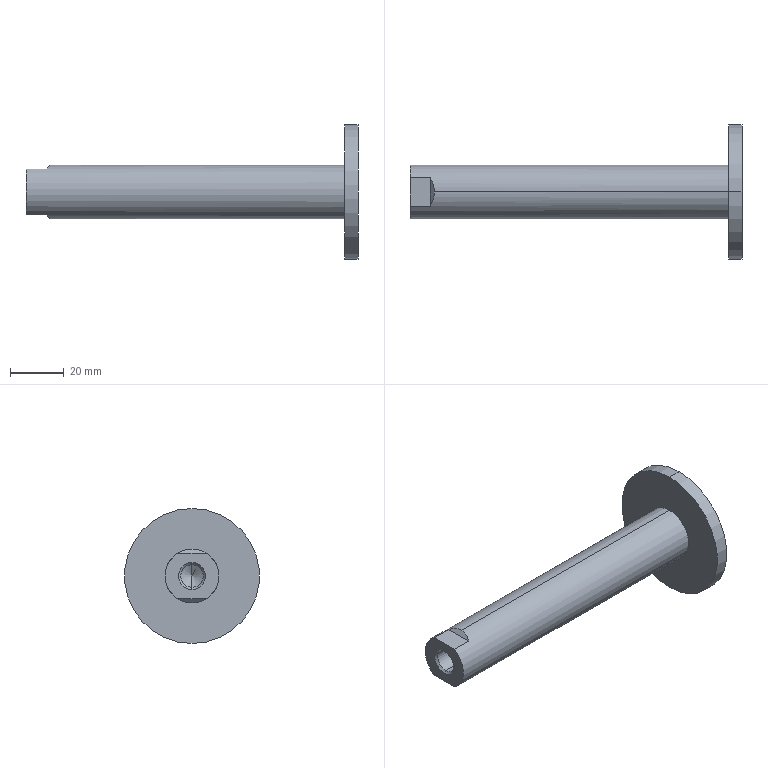Part | STEP file | _CDQ2A50-100-D-A93(0_0)_CYROD.stp | 1 solid | 17 faces | box 123 x 50 x 50 mm | volume 45835 mm3 | plane 7 | cylinder 6 | cone 4 | commonest cylinder face diameters 8.376 x2 20 x2 50 x2
STEP:
#1=CARTESIAN_POINT('',(0.,0.,0.));
#2=DIRECTION('',(0.,0.,1.));
#3=DIRECTION('',(1.,0.,0.));
#4=AXIS2_PLACEMENT_3D('',#1,#2,#3);
#5=CARTESIAN_POINT('',(7.,0.,4.188));
#6=VERTEX_POINT('',#5);
#7=CARTESIAN_POINT('',(7.,0.,-4.188));
#8=VERTEX_POINT('',#7);
#9=CARTESIAN_POINT('',(7.,0.,0.));
#10=DIRECTION('',(1.,0.,0.));
#11=DIRECTION('',(0.,0.,-1.));
#12=AXIS2_PLACEMENT_3D('',#9,#10,#11);
#13=CIRCLE('',#12,4.188);
#14=CARTESIAN_POINT('',(8.418,0.,0.));
#15=DIRECTION('',(-1.,0.,0.));
#16=DIRECTION('',(0.,0.,1.));
#17=AXIS2_PLACEMENT_3D('',#14,#15,#16);
#18=CONICAL_SURFACE('',#17,1.732,1.047);
#19=CARTESIAN_POINT('',(9.425,1.418));
#20=DIRECTION('',(-1.,0.));
#21=VECTOR('',#20,1.);
#22=LINE('',#19,#21);
#23=(GEOMETRIC_REPRESENTATION_CONTEXT(2)PARAMETRIC_REPRESENTATION_CONTEXT()REPRESENTATION_CONTEXT('',''));
#24=DEFINITIONAL_REPRESENTATION('',(#22),#23);
#25=PCURVE('',#18,#24);
#26=CARTESIAN_POINT('',(115.,0.,0.));
#27=DIRECTION('',(-1.,0.,0.));
#28=DIRECTION('',(0.,0.,-1.));
#29=AXIS2_PLACEMENT_3D('',#26,#27,#28);
#30=CYLINDRICAL_SURFACE('',#29,4.188);
#31=CARTESIAN_POINT('',(6.283,108.));
#32=DIRECTION('',(-1.,0.));
#33=VECTOR('',#32,1.);
#34=LINE('',#31,#33);
#35=(GEOMETRIC_REPRESENTATION_CONTEXT(2)PARAMETRIC_REPRESENTATION_CONTEXT()REPRESENTATION_CONTEXT('',''));
#36=DEFINITIONAL_REPRESENTATION('',(#34),#35);
#37=PCURVE('',#30,#36);
#38=SURFACE_CURVE('',#13,(#25,#37),.PCURVE_S1.);
#39=EDGE_CURVE('',#6,#8,#38,.T.);
#40=ORIENTED_EDGE('',*,*,#39,.T.);
#41=CARTESIAN_POINT('',(9.418,0.,0.));
#42=VERTEX_POINT('',#41);
#43=CARTESIAN_POINT('',(8.418,0.,-1.732));
#44=DIRECTION('',(-0.5,0.,-0.866));
#45=VECTOR('',#44,1.);
#46=LINE('',#43,#45);
#47=CARTESIAN_POINT('',(3.142,0.));
#48=DIRECTION('',(0.,1.));
#49=VECTOR('',#48,1.);
#50=LINE('',#47,#49);
#51=(GEOMETRIC_REPRESENTATION_CONTEXT(2)PARAMETRIC_REPRESENTATION_CONTEXT()REPRESENTATION_CONTEXT('',''));
#52=DEFINITIONAL_REPRESENTATION('',(#50),#51);
#53=PCURVE('',#18,#52);
#54=CARTESIAN_POINT('',(8.418,0.,0.));
#55=DIRECTION('',(-1.,0.,0.));
#56=DIRECTION('',(0.,0.,1.));
#57=AXIS2_PLACEMENT_3D('',#54,#55,#56);
#58=CONICAL_SURFACE('',#57,1.732,1.047);
#59=CARTESIAN_POINT('',(3.142,0.));
#60=DIRECTION('',(0.,1.));
#61=VECTOR('',#60,1.);
#62=LINE('',#59,#61);
#63=(GEOMETRIC_REPRESENTATION_CONTEXT(2)PARAMETRIC_REPRESENTATION_CONTEXT()REPRESENTATION_CONTEXT('',''));
#64=DEFINITIONAL_REPRESENTATION('',(#62),#63);
#65=PCURVE('',#58,#64);
#66=SURFACE_CURVE('',#46,(#53,#65),.PCURVE_S1.);
#67=EDGE_CURVE('',#42,#8,#66,.T.);
#68=ORIENTED_EDGE('',*,*,#67,.F.);
#69=CARTESIAN_POINT('',(8.418,0.,1.732));
#70=DIRECTION('',(-0.5,0.,0.866));
#71=VECTOR('',#70,1.);
#72=LINE('',#69,#71);
#73=CARTESIAN_POINT('',(6.283,0.));
#74=DIRECTION('',(0.,1.));
#75=VECTOR('',#74,1.);
#76=LINE('',#73,#75);
#77=(GEOMETRIC_REPRESENTATION_CONTEXT(2)PARAMETRIC_REPRESENTATION_CONTEXT()REPRESENTATION_CONTEXT('',''));
#78=DEFINITIONAL_REPRESENTATION('',(#76),#77);
#79=PCURVE('',#18,#78);
#80=CARTESIAN_POINT('',(0.,0.));
#81=DIRECTION('',(0.,1.));
#82=VECTOR('',#81,1.);
#83=LINE('',#80,#82);
#84=(GEOMETRIC_REPRESENTATION_CONTEXT(2)PARAMETRIC_REPRESENTATION_CONTEXT()REPRESENTATION_CONTEXT('',''));
#85=DEFINITIONAL_REPRESENTATION('',(#83),#84);
#86=PCURVE('',#58,#85);
#87=SURFACE_CURVE('',#72,(#79,#86),.PCURVE_S1.);
#88=EDGE_CURVE('',#42,#6,#87,.T.);
#89=ORIENTED_EDGE('',*,*,#88,.T.);
#90=EDGE_LOOP('',(#40,#68,#89));
#91=FACE_BOUND('',#90,.F.);
#92=ADVANCED_FACE('',(#91),#18,.F.);
#93=CARTESIAN_POINT('',(-0.5,5.268,-8.5));
#94=VERTEX_POINT('',#93);
#95=CARTESIAN_POINT('',(1.,0.,-10.));
#96=VERTEX_POINT('',#95);
#97=CARTESIAN_POINT('',(-0.5,5.268,-8.5));
#98=CARTESIAN_POINT('',(0.4869,3.675,-9.487));
#99=CARTESIAN_POINT('',(1.,1.873,-10.));
#100=CARTESIAN_POINT('',(1.,0.,-10.));
#101=(BOUNDED_CURVE()B_SPLINE_CURVE(3,(#97,#98,#99,#100),.UNSPECIFIED.,.F.,.F.)B_SPLINE_CURVE_WITH_KNOTS((4,4),(5.728,6.283),.PIECEWISE_BEZIER_KNOTS.)CURVE()GEOMETRIC_REPRESENTATION_ITEM()RATIONAL_B_SPLINE_CURVE((1.,0.9745,0.9745,1.))REPRESENTATION_ITEM(''));
#102=CARTESIAN_POINT('',(1.055,-5.795,-10.055));
#103=DIRECTION('',(-0.7071,0.,-0.7071));
#104=DIRECTION('',(-0.7071,0.,0.7071));
#105=AXIS2_PLACEMENT_3D('',#102,#103,#104);
#106=PLANE('',#105);
#107=CARTESIAN_POINT('',(2.199,11.062));
#108=CARTESIAN_POINT('',(0.8035,9.47));
#109=CARTESIAN_POINT('',(0.07786,7.668));
#110=CARTESIAN_POINT('',(0.07786,5.795));
#111=(BOUNDED_CURVE()B_SPLINE_CURVE(3,(#107,#108,#109,#110),.UNSPECIFIED.,.F.,.F.)B_SPLINE_CURVE_WITH_KNOTS((4,4),(5.728,6.283),.PIECEWISE_BEZIER_KNOTS.)CURVE()GEOMETRIC_REPRESENTATION_ITEM()RATIONAL_B_SPLINE_CURVE((1.,0.9745,0.9745,1.))REPRESENTATION_ITEM(''));
#112=(GEOMETRIC_REPRESENTATION_CONTEXT(2)PARAMETRIC_REPRESENTATION_CONTEXT()REPRESENTATION_CONTEXT('',''));
#113=DEFINITIONAL_REPRESENTATION('',(#111),#112);
#114=PCURVE('',#106,#113);
#115=CARTESIAN_POINT('',(115.,0.,0.));
#116=DIRECTION('',(-1.,0.,0.));
#117=DIRECTION('',(0.,0.,-1.));
#118=AXIS2_PLACEMENT_3D('',#115,#116,#117);
#119=CYLINDRICAL_SURFACE('',#118,10.);
#120=CARTESIAN_POINT('',(5.728,115.5));
#121=CARTESIAN_POINT('',(5.737,115.456));
#122=CARTESIAN_POINT('',(5.753,115.37));
#123=CARTESIAN_POINT('',(5.778,115.247));
#124=CARTESIAN_POINT('',(5.803,115.128));
#125=CARTESIAN_POINT('',(5.829,115.015));
#126=CARTESIAN_POINT('',(5.854,114.907));
#127=CARTESIAN_POINT('',(5.879,114.805));
#128=CARTESIAN_POINT('',(5.904,114.708));
#129=CARTESIAN_POINT('',(5.93,114.617));
#130=CARTESIAN_POINT('',(5.955,114.533));
#131=CARTESIAN_POINT('',(5.98,114.454));
#132=CARTESIAN_POINT('',(6.006,114.381));
#133=CARTESIAN_POINT('',(6.031,114.315));
#134=CARTESIAN_POINT('',(6.057,114.255));
#135=CARTESIAN_POINT('',(6.082,114.201));
#136=CARTESIAN_POINT('',(6.107,114.153));
#137=CARTESIAN_POINT('',(6.133,114.112));
#138=CARTESIAN_POINT('',(6.158,114.077));
#139=CARTESIAN_POINT('',(6.183,114.049));
#140=CARTESIAN_POINT('',(6.208,114.027));
#141=CARTESIAN_POINT('',(6.233,114.011));
#142=CARTESIAN_POINT('',(6.258,114.002));
#143=CARTESIAN_POINT('',(6.275,114.));
#144=CARTESIAN_POINT('',(6.283,114.));
#145=B_SPLINE_CURVE_WITH_KNOTS('',3,(#120,#121,#122,#123,#124,#125,#126,#127,#128,#129,#130,#131,#132,#133,#134,#135,#136,#137,#138,#139,#140,#141,#142,#143,#144),.UNSPECIFIED.,.F.,.F.,(4,1,1,1,1,1,1,1,1,1,1,1,1,1,1,1,1,1,1,1,1,1,4),(5.728,5.754,5.779,5.804,5.829,5.854,5.88,5.905,5.93,5.955,5.981,6.006,6.031,6.056,6.081,6.107,6.132,6.157,6.182,6.208,6.233,6.258,6.283),.QUASI_UNIFORM_KNOTS.);
#146=(GEOMETRIC_REPRESENTATION_CONTEXT(2)PARAMETRIC_REPRESENTATION_CONTEXT()REPRESENTATION_CONTEXT('',''));
#147=DEFINITIONAL_REPRESENTATION('',(#145),#146);
#148=PCURVE('',#119,#147);
#149=SURFACE_CURVE('',#101,(#114,#148),.PCURVE_S1.);
#150=EDGE_CURVE('',#94,#96,#149,.T.);
#151=ORIENTED_EDGE('',*,*,#150,.T.);
#152=CARTESIAN_POINT('',(-0.5,-5.268,-8.5));
#153=VERTEX_POINT('',#152);
#154=CARTESIAN_POINT('',(1.,0.,-10.));
#155=CARTESIAN_POINT('',(1.,-1.873,-10.));
#156=CARTESIAN_POINT('',(0.4869,-3.675,-9.487));
#157=CARTESIAN_POINT('',(-0.5,-5.268,-8.5));
#158=(BOUNDED_CURVE()B_SPLINE_CURVE(3,(#154,#155,#156,#157),.UNSPECIFIED.,.F.,.F.)B_SPLINE_CURVE_WITH_KNOTS((4,4),(0.,0.5548),.PIECEWISE_BEZIER_KNOTS.)CURVE()GEOMETRIC_REPRESENTATION_ITEM()RATIONAL_B_SPLINE_CURVE((1.,0.9745,0.9745,1.))REPRESENTATION_ITEM(''));
#159=CARTESIAN_POINT('',(0.07786,5.795));
#160=CARTESIAN_POINT('',(0.07786,3.921));
#161=CARTESIAN_POINT('',(0.8035,2.119));
#162=CARTESIAN_POINT('',(2.199,0.5268));
#163=(BOUNDED_CURVE()B_SPLINE_CURVE(3,(#159,#160,#161,#162),.UNSPECIFIED.,.F.,.F.)B_SPLINE_CURVE_WITH_KNOTS((4,4),(0.,0.5548),.PIECEWISE_BEZIER_KNOTS.)CURVE()GEOMETRIC_REPRESENTATION_ITEM()RATIONAL_B_SPLINE_CURVE((1.,0.9745,0.9745,1.))REPRESENTATION_ITEM(''));
#164=(GEOMETRIC_REPRESENTATION_CONTEXT(2)PARAMETRIC_REPRESENTATION_CONTEXT()REPRESENTATION_CONTEXT('',''));
#165=DEFINITIONAL_REPRESENTATION('',(#163),#164);
#166=PCURVE('',#106,#165);
#167=CARTESIAN_POINT('',(115.,0.,0.));
#168=DIRECTION('',(-1.,0.,0.));
#169=DIRECTION('',(0.,0.,-1.));
#170=AXIS2_PLACEMENT_3D('',#167,#168,#169);
#171=CYLINDRICAL_SURFACE('',#170,10.);
#172=CARTESIAN_POINT('',(0.,114.));
#173=CARTESIAN_POINT('',(0.008299,114.));
#174=CARTESIAN_POINT('',(0.02493,114.002));
#175=CARTESIAN_POINT('',(0.04994,114.011));
#176=CARTESIAN_POINT('',(0.07503,114.027));
#177=CARTESIAN_POINT('',(0.1002,114.049));
#178=CARTESIAN_POINT('',(0.1254,114.077));
#179=CARTESIAN_POINT('',(0.1507,114.112));
#180=CARTESIAN_POINT('',(0.176,114.153));
#181=CARTESIAN_POINT('',(0.2013,114.201));
#182=CARTESIAN_POINT('',(0.2267,114.255));
#183=CARTESIAN_POINT('',(0.252,114.315));
#184=CARTESIAN_POINT('',(0.2774,114.381));
#185=CARTESIAN_POINT('',(0.3028,114.454));
#186=CARTESIAN_POINT('',(0.3282,114.533));
#187=CARTESIAN_POINT('',(0.3535,114.617));
#188=CARTESIAN_POINT('',(0.3789,114.708));
#189=CARTESIAN_POINT('',(0.4042,114.805));
#190=CARTESIAN_POINT('',(0.4294,114.907));
#191=CARTESIAN_POINT('',(0.4546,115.015));
#192=CARTESIAN_POINT('',(0.4798,115.128));
#193=CARTESIAN_POINT('',(0.5049,115.247));
#194=CARTESIAN_POINT('',(0.5299,115.37));
#195=CARTESIAN_POINT('',(0.5465,115.456));
#196=CARTESIAN_POINT('',(0.5548,115.5));
#197=B_SPLINE_CURVE_WITH_KNOTS('',3,(#172,#173,#174,#175,#176,#177,#178,#179,#180,#181,#182,#183,#184,#185,#186,#187,#188,#189,#190,#191,#192,#193,#194,#195,#196),.UNSPECIFIED.,.F.,.F.,(4,1,1,1,1,1,1,1,1,1,1,1,1,1,1,1,1,1,1,1,1,1,4),(0.,0.02522,0.05044,0.07566,0.1009,0.1261,0.1513,0.1765,0.2017,0.227,0.2522,0.2774,0.3026,0.3278,0.3531,0.3783,0.4035,0.4287,0.4539,0.4792,0.5044,0.5296,0.5548),.QUASI_UNIFORM_KNOTS.);
#198=(GEOMETRIC_REPRESENTATION_CONTEXT(2)PARAMETRIC_REPRESENTATION_CONTEXT()REPRESENTATION_CONTEXT('',''));
#199=DEFINITIONAL_REPRESENTATION('',(#197),#198);
#200=PCURVE('',#171,#199);
#201=SURFACE_CURVE('',#158,(#166,#200),.PCURVE_S1.);
#202=EDGE_CURVE('',#96,#153,#201,.T.);
#203=ORIENTED_EDGE('',*,*,#202,.T.);
#204=CARTESIAN_POINT('',(-0.5,5.268,-8.5));
#205=DIRECTION('',(0.,-1.,0.));
#206=VECTOR('',#205,1.);
#207=LINE('',#204,#206);
#208=CARTESIAN_POINT('',(2.199,11.062));
#209=DIRECTION('',(0.,-1.));
#210=VECTOR('',#209,1.);
#211=LINE('',#208,#210);
#212=(GEOMETRIC_REPRESENTATION_CONTEXT(2)PARAMETRIC_REPRESENTATION_CONTEXT()REPRESENTATION_CONTEXT('',''));
#213=DEFINITIONAL_REPRESENTATION('',(#211),#212);
#214=PCURVE('',#106,#213);
#215=CARTESIAN_POINT('',(-0.125,-5.795,-8.5));
#216=DIRECTION('',(0.,0.,-1.));
#217=DIRECTION('',(0.,-1.,0.));
#218=AXIS2_PLACEMENT_3D('',#215,#216,#217);
#219=PLANE('',#218);
#220=CARTESIAN_POINT('',(-11.062,0.375));
#221=DIRECTION('',(1.,0.));
#222=VECTOR('',#221,1.);
#223=LINE('',#220,#222);
#224=(GEOMETRIC_REPRESENTATION_CONTEXT(2)PARAMETRIC_REPRESENTATION_CONTEXT()REPRESENTATION_CONTEXT('',''));
#225=DEFINITIONAL_REPRESENTATION('',(#223),#224);
#226=PCURVE('',#219,#225);
#227=SURFACE_CURVE('',#207,(#214,#226),.PCURVE_S1.);
#228=EDGE_CURVE('',#94,#153,#227,.T.);
#229=ORIENTED_EDGE('',*,*,#228,.F.);
#230=EDGE_LOOP('',(#151,#203,#229));
#231=FACE_BOUND('',#230,.T.);
#232=ADVANCED_FACE('',(#231),#106,.T.);
#233=CARTESIAN_POINT('',(-8.,5.268,-8.5));
#234=VERTEX_POINT('',#233);
#235=CARTESIAN_POINT('',(-8.,5.268,-8.5));
#236=DIRECTION('',(1.,0.,0.));
#237=VECTOR('',#236,1.);
#238=LINE('',#235,#237);
#239=CARTESIAN_POINT('',(-11.062,7.875));
#240=DIRECTION('',(0.,-1.));
#241=VECTOR('',#240,1.);
#242=LINE('',#239,#241);
#243=(GEOMETRIC_REPRESENTATION_CONTEXT(2)PARAMETRIC_REPRESENTATION_CONTEXT()REPRESENTATION_CONTEXT('',''));
#244=DEFINITIONAL_REPRESENTATION('',(#242),#243);
#245=PCURVE('',#219,#244);
#246=CARTESIAN_POINT('',(5.728,123.));
#247=DIRECTION('',(0.,-1.));
#248=VECTOR('',#247,1.);
#249=LINE('',#246,#248);
#250=(GEOMETRIC_REPRESENTATION_CONTEXT(2)PARAMETRIC_REPRESENTATION_CONTEXT()REPRESENTATION_CONTEXT('',''));
#251=DEFINITIONAL_REPRESENTATION('',(#249),#250);
#252=PCURVE('',#119,#251);
#253=SURFACE_CURVE('',#238,(#245,#252),.PCURVE_S1.);
#254=EDGE_CURVE('',#234,#94,#253,.T.);
#255=ORIENTED_EDGE('',*,*,#254,.T.);
#256=ORIENTED_EDGE('',*,*,#228,.T.);
#257=CARTESIAN_POINT('',(-8.,-5.268,-8.5));
#258=VERTEX_POINT('',#257);
#259=CARTESIAN_POINT('',(-8.,-5.268,-8.5));
#260=DIRECTION('',(-1.,0.,0.));
#261=VECTOR('',#260,1.);
#262=LINE('',#259,#261);
#263=CARTESIAN_POINT('',(-0.5268,7.875));
#264=DIRECTION('',(0.,1.));
#265=VECTOR('',#264,1.);
#266=LINE('',#263,#265);
#267=(GEOMETRIC_REPRESENTATION_CONTEXT(2)PARAMETRIC_REPRESENTATION_CONTEXT()REPRESENTATION_CONTEXT('',''));
#268=DEFINITIONAL_REPRESENTATION('',(#266),#267);
#269=PCURVE('',#219,#268);
#270=CARTESIAN_POINT('',(0.5548,123.));
#271=DIRECTION('',(0.,1.));
#272=VECTOR('',#271,1.);
#273=LINE('',#270,#272);
#274=(GEOMETRIC_REPRESENTATION_CONTEXT(2)PARAMETRIC_REPRESENTATION_CONTEXT()REPRESENTATION_CONTEXT('',''));
#275=DEFINITIONAL_REPRESENTATION('',(#273),#274);
#276=PCURVE('',#171,#275);
#277=SURFACE_CURVE('',#262,(#269,#276),.PCURVE_S1.);
#278=EDGE_CURVE('',#153,#258,#277,.T.);
#279=ORIENTED_EDGE('',*,*,#278,.T.);
#280=CARTESIAN_POINT('',(-8.,5.268,-8.5));
#281=DIRECTION('',(0.,-1.,0.));
#282=VECTOR('',#281,1.);
#283=LINE('',#280,#282);
#284=CARTESIAN_POINT('',(-11.062,7.875));
#285=DIRECTION('',(1.,0.));
#286=VECTOR('',#285,1.);
#287=LINE('',#284,#286);
#288=(GEOMETRIC_REPRESENTATION_CONTEXT(2)PARAMETRIC_REPRESENTATION_CONTEXT()REPRESENTATION_CONTEXT('',''));
#289=DEFINITIONAL_REPRESENTATION('',(#287),#288);
#290=PCURVE('',#219,#289);
#291=CARTESIAN_POINT('',(-8.,-11.,9.35));
#292=DIRECTION('',(1.,0.,0.));
#293=DIRECTION('',(0.,1.,0.));
#294=AXIS2_PLACEMENT_3D('',#291,#292,#293);
#295=PLANE('',#294);
#296=CARTESIAN_POINT('',(16.268,-17.85));
#297=DIRECTION('',(-1.,0.));
#298=VECTOR('',#297,1.);
#299=LINE('',#296,#298);
#300=(GEOMETRIC_REPRESENTATION_CONTEXT(2)PARAMETRIC_REPRESENTATION_CONTEXT()REPRESENTATION_CONTEXT('',''));
#301=DEFINITIONAL_REPRESENTATION('',(#299),#300);
#302=PCURVE('',#295,#301);
#303=SURFACE_CURVE('',#283,(#290,#302),.PCURVE_S1.);
#304=EDGE_CURVE('',#234,#258,#303,.T.);
#305=ORIENTED_EDGE('',*,*,#304,.F.);
#306=EDGE_LOOP('',(#255,#256,#279,#305));
#307=FACE_BOUND('',#306,.T.);
#308=ADVANCED_FACE('',(#307),#219,.T.);
#309=CARTESIAN_POINT('',(-8.,-5.268,8.5));
#310=VERTEX_POINT('',#309);
#311=CARTESIAN_POINT('',(-0.5,-5.268,8.5));
#312=VERTEX_POINT('',#311);
#313=CARTESIAN_POINT('',(-8.,-5.268,8.5));
#314=DIRECTION('',(1.,0.,0.));
#315=VECTOR('',#314,1.);
#316=LINE('',#313,#315);
#317=CARTESIAN_POINT('',(-8.375,-5.795,8.5));
#318=DIRECTION('',(0.,0.,1.));
#319=DIRECTION('',(1.,0.,0.));
#320=AXIS2_PLACEMENT_3D('',#317,#318,#319);
#321=PLANE('',#320);
#322=CARTESIAN_POINT('',(0.375,0.5268));
#323=DIRECTION('',(1.,0.));
#324=VECTOR('',#323,1.);
#325=LINE('',#322,#324);
#326=(GEOMETRIC_REPRESENTATION_CONTEXT(2)PARAMETRIC_REPRESENTATION_CONTEXT()REPRESENTATION_CONTEXT('',''));
#327=DEFINITIONAL_REPRESENTATION('',(#325),#326);
#328=PCURVE('',#321,#327);
#329=CARTESIAN_POINT('',(2.587,123.));
#330=DIRECTION('',(0.,-1.));
#331=VECTOR('',#330,1.);
#332=LINE('',#329,#331);
#333=(GEOMETRIC_REPRESENTATION_CONTEXT(2)PARAMETRIC_REPRESENTATION_CONTEXT()REPRESENTATION_CONTEXT('',''));
#334=DEFINITIONAL_REPRESENTATION('',(#332),#333);
#335=PCURVE('',#171,#334);
#336=SURFACE_CURVE('',#316,(#328,#335),.PCURVE_S1.);
#337=EDGE_CURVE('',#310,#312,#336,.T.);
#338=ORIENTED_EDGE('',*,*,#337,.T.);
#339=CARTESIAN_POINT('',(-0.5,5.268,8.5));
#340=VERTEX_POINT('',#339);
#341=CARTESIAN_POINT('',(-0.5,5.268,8.5));
#342=DIRECTION('',(0.,-1.,0.));
#343=VECTOR('',#342,1.);
#344=LINE('',#341,#343);
#345=CARTESIAN_POINT('',(7.875,11.062));
#346=DIRECTION('',(0.,-1.));
#347=VECTOR('',#346,1.);
#348=LINE('',#345,#347);
#349=(GEOMETRIC_REPRESENTATION_CONTEXT(2)PARAMETRIC_REPRESENTATION_CONTEXT()REPRESENTATION_CONTEXT('',''));
#350=DEFINITIONAL_REPRESENTATION('',(#348),#349);
#351=PCURVE('',#321,#350);
#352=CARTESIAN_POINT('',(-0.5741,-5.795,8.426));
#353=DIRECTION('',(-0.7071,0.,0.7071));
#354=DIRECTION('',(0.,1.,0.));
#355=AXIS2_PLACEMENT_3D('',#352,#353,#354);
#356=PLANE('',#355);
#357=CARTESIAN_POINT('',(11.062,-0.1047));
#358=DIRECTION('',(-1.,0.));
#359=VECTOR('',#358,1.);
#360=LINE('',#357,#359);
#361=(GEOMETRIC_REPRESENTATION_CONTEXT(2)PARAMETRIC_REPRESENTATION_CONTEXT()REPRESENTATION_CONTEXT('',''));
#362=DEFINITIONAL_REPRESENTATION('',(#360),#361);
#363=PCURVE('',#356,#362);
#364=SURFACE_CURVE('',#344,(#351,#363),.PCURVE_S1.);
#365=EDGE_CURVE('',#340,#312,#364,.T.);
#366=ORIENTED_EDGE('',*,*,#365,.F.);
#367=CARTESIAN_POINT('',(-8.,5.268,8.5));
#368=VERTEX_POINT('',#367);
#369=CARTESIAN_POINT('',(-8.,5.268,8.5));
#370=DIRECTION('',(-1.,0.,0.));
#371=VECTOR('',#370,1.);
#372=LINE('',#369,#371);
#373=CARTESIAN_POINT('',(0.375,11.062));
#374=DIRECTION('',(-1.,0.));
#375=VECTOR('',#374,1.);
#376=LINE('',#373,#375);
#377=(GEOMETRIC_REPRESENTATION_CONTEXT(2)PARAMETRIC_REPRESENTATION_CONTEXT()REPRESENTATION_CONTEXT('',''));
#378=DEFINITIONAL_REPRESENTATION('',(#376),#377);
#379=PCURVE('',#321,#378);
#380=CARTESIAN_POINT('',(3.696,123.));
#381=DIRECTION('',(0.,1.));
#382=VECTOR('',#381,1.);
#383=LINE('',#380,#382);
#384=(GEOMETRIC_REPRESENTATION_CONTEXT(2)PARAMETRIC_REPRESENTATION_CONTEXT()REPRESENTATION_CONTEXT('',''));
#385=DEFINITIONAL_REPRESENTATION('',(#383),#384);
#386=PCURVE('',#119,#385);
#387=SURFACE_CURVE('',#372,(#379,#386),.PCURVE_S1.);
#388=EDGE_CURVE('',#340,#368,#387,.T.);
#389=ORIENTED_EDGE('',*,*,#388,.T.);
#390=CARTESIAN_POINT('',(-8.,5.268,8.5));
#391=DIRECTION('',(0.,-1.,0.));
#392=VECTOR('',#391,1.);
#393=LINE('',#390,#392);
#394=CARTESIAN_POINT('',(0.375,11.062));
#395=DIRECTION('',(0.,-1.));
#396=VECTOR('',#395,1.);
#397=LINE('',#394,#396);
#398=(GEOMETRIC_REPRESENTATION_CONTEXT(2)PARAMETRIC_REPRESENTATION_CONTEXT()REPRESENTATION_CONTEXT('',''));
#399=DEFINITIONAL_REPRESENTATION('',(#397),#398);
#400=PCURVE('',#321,#399);
#401=CARTESIAN_POINT('',(16.268,-0.85));
#402=DIRECTION('',(-1.,0.));
#403=VECTOR('',#402,1.);
#404=LINE('',#401,#403);
#405=(GEOMETRIC_REPRESENTATION_CONTEXT(2)PARAMETRIC_REPRESENTATION_CONTEXT()REPRESENTATION_CONTEXT('',''));
#406=DEFINITIONAL_REPRESENTATION('',(#404),#405);
#407=PCURVE('',#295,#406);
#408=SURFACE_CURVE('',#393,(#400,#407),.PCURVE_S1.);
#409=EDGE_CURVE('',#368,#310,#408,.T.);
#410=ORIENTED_EDGE('',*,*,#409,.T.);
#411=EDGE_LOOP('',(#338,#366,#389,#410));
#412=FACE_BOUND('',#411,.T.);
#413=ADVANCED_FACE('',(#412),#321,.T.);
#414=CARTESIAN_POINT('',(1.,0.,10.));
#415=VERTEX_POINT('',#414);
#416=CARTESIAN_POINT('',(-0.5,-5.268,8.5));
#417=CARTESIAN_POINT('',(0.4869,-3.675,9.487));
#418=CARTESIAN_POINT('',(1.,-1.873,10.));
#419=CARTESIAN_POINT('',(1.,0.,10.));
#420=(BOUNDED_CURVE()B_SPLINE_CURVE(3,(#416,#417,#418,#419),.UNSPECIFIED.,.F.,.F.)B_SPLINE_CURVE_WITH_KNOTS((4,4),(5.728,6.283),.PIECEWISE_BEZIER_KNOTS.)CURVE()GEOMETRIC_REPRESENTATION_ITEM()RATIONAL_B_SPLINE_CURVE((1.,0.9745,0.9745,1.))REPRESENTATION_ITEM(''));
#421=CARTESIAN_POINT('',(0.5268,-0.1047));
#422=CARTESIAN_POINT('',(2.119,-1.5));
#423=CARTESIAN_POINT('',(3.921,-2.226));
#424=CARTESIAN_POINT('',(5.795,-2.226));
#425=(BOUNDED_CURVE()B_SPLINE_CURVE(3,(#421,#422,#423,#424),.UNSPECIFIED.,.F.,.F.)B_SPLINE_CURVE_WITH_KNOTS((4,4),(5.728,6.283),.PIECEWISE_BEZIER_KNOTS.)CURVE()GEOMETRIC_REPRESENTATION_ITEM()RATIONAL_B_SPLINE_CURVE((1.,0.9745,0.9745,1.))REPRESENTATION_ITEM(''));
#426=(GEOMETRIC_REPRESENTATION_CONTEXT(2)PARAMETRIC_REPRESENTATION_CONTEXT()REPRESENTATION_CONTEXT('',''));
#427=DEFINITIONAL_REPRESENTATION('',(#425),#426);
#428=PCURVE('',#356,#427);
#429=CARTESIAN_POINT('',(2.587,115.5));
#430=CARTESIAN_POINT('',(2.595,115.456));
#431=CARTESIAN_POINT('',(2.612,115.37));
#432=CARTESIAN_POINT('',(2.637,115.247));
#433=CARTESIAN_POINT('',(2.662,115.128));
#434=CARTESIAN_POINT('',(2.687,115.015));
#435=CARTESIAN_POINT('',(2.712,114.907));
#436=CARTESIAN_POINT('',(2.737,114.805));
#437=CARTESIAN_POINT('',(2.763,114.708));
#438=CARTESIAN_POINT('',(2.788,114.617));
#439=CARTESIAN_POINT('',(2.813,114.533));
#440=CARTESIAN_POINT('',(2.839,114.454));
#441=CARTESIAN_POINT('',(2.864,114.381));
#442=CARTESIAN_POINT('',(2.89,114.315));
#443=CARTESIAN_POINT('',(2.915,114.255));
#444=CARTESIAN_POINT('',(2.94,114.201));
#445=CARTESIAN_POINT('',(2.966,114.153));
#446=CARTESIAN_POINT('',(2.991,114.112));
#447=CARTESIAN_POINT('',(3.016,114.077));
#448=CARTESIAN_POINT('',(3.041,114.049));
#449=CARTESIAN_POINT('',(3.067,114.027));
#450=CARTESIAN_POINT('',(3.092,114.011));
#451=CARTESIAN_POINT('',(3.117,114.002));
#452=CARTESIAN_POINT('',(3.133,114.));
#453=CARTESIAN_POINT('',(3.142,114.));
#454=B_SPLINE_CURVE_WITH_KNOTS('',3,(#429,#430,#431,#432,#433,#434,#435,#436,#437,#438,#439,#440,#441,#442,#443,#444,#445,#446,#447,#448,#449,#450,#451,#452,#453),.UNSPECIFIED.,.F.,.F.,(4,1,1,1,1,1,1,1,1,1,1,1,1,1,1,1,1,1,1,1,1,1,4),(5.728,5.754,5.779,5.804,5.829,5.854,5.88,5.905,5.93,5.955,5.981,6.006,6.031,6.056,6.081,6.107,6.132,6.157,6.182,6.208,6.233,6.258,6.283),.QUASI_UNIFORM_KNOTS.);
#455=(GEOMETRIC_REPRESENTATION_CONTEXT(2)PARAMETRIC_REPRESENTATION_CONTEXT()REPRESENTATION_CONTEXT('',''));
#456=DEFINITIONAL_REPRESENTATION('',(#454),#455);
#457=PCURVE('',#171,#456);
#458=SURFACE_CURVE('',#420,(#428,#457),.PCURVE_S1.);
#459=EDGE_CURVE('',#312,#415,#458,.T.);
#460=ORIENTED_EDGE('',*,*,#459,.T.);
#461=CARTESIAN_POINT('',(1.,0.,10.));
#462=CARTESIAN_POINT('',(1.,1.873,10.));
#463=CARTESIAN_POINT('',(0.4869,3.675,9.487));
#464=CARTESIAN_POINT('',(-0.5,5.268,8.5));
#465=(BOUNDED_CURVE()B_SPLINE_CURVE(3,(#461,#462,#463,#464),.UNSPECIFIED.,.F.,.F.)B_SPLINE_CURVE_WITH_KNOTS((4,4),(0.,0.5548),.PIECEWISE_BEZIER_KNOTS.)CURVE()GEOMETRIC_REPRESENTATION_ITEM()RATIONAL_B_SPLINE_CURVE((1.,0.9745,0.9745,1.))REPRESENTATION_ITEM(''));
#466=CARTESIAN_POINT('',(5.795,-2.226));
#467=CARTESIAN_POINT('',(7.668,-2.226));
#468=CARTESIAN_POINT('',(9.47,-1.5));
#469=CARTESIAN_POINT('',(11.062,-0.1047));
#470=(BOUNDED_CURVE()B_SPLINE_CURVE(3,(#466,#467,#468,#469),.UNSPECIFIED.,.F.,.F.)B_SPLINE_CURVE_WITH_KNOTS((4,4),(0.,0.5548),.PIECEWISE_BEZIER_KNOTS.)CURVE()GEOMETRIC_REPRESENTATION_ITEM()RATIONAL_B_SPLINE_CURVE((1.,0.9745,0.9745,1.))REPRESENTATION_ITEM(''));
#471=(GEOMETRIC_REPRESENTATION_CONTEXT(2)PARAMETRIC_REPRESENTATION_CONTEXT()REPRESENTATION_CONTEXT('',''));
#472=DEFINITIONAL_REPRESENTATION('',(#470),#471);
#473=PCURVE('',#356,#472);
#474=CARTESIAN_POINT('',(3.142,114.));
#475=CARTESIAN_POINT('',(3.15,114.));
#476=CARTESIAN_POINT('',(3.167,114.002));
#477=CARTESIAN_POINT('',(3.192,114.011));
#478=CARTESIAN_POINT('',(3.217,114.027));
#479=CARTESIAN_POINT('',(3.242,114.049));
#480=CARTESIAN_POINT('',(3.267,114.077));
#481=CARTESIAN_POINT('',(3.292,114.112));
#482=CARTESIAN_POINT('',(3.318,114.153));
#483=CARTESIAN_POINT('',(3.343,114.201));
#484=CARTESIAN_POINT('',(3.368,114.255));
#485=CARTESIAN_POINT('',(3.394,114.315));
#486=CARTESIAN_POINT('',(3.419,114.381));
#487=CARTESIAN_POINT('',(3.444,114.454));
#488=CARTESIAN_POINT('',(3.47,114.533));
#489=CARTESIAN_POINT('',(3.495,114.617));
#490=CARTESIAN_POINT('',(3.52,114.708));
#491=CARTESIAN_POINT('',(3.546,114.805));
#492=CARTESIAN_POINT('',(3.571,114.907));
#493=CARTESIAN_POINT('',(3.596,115.015));
#494=CARTESIAN_POINT('',(3.621,115.128));
#495=CARTESIAN_POINT('',(3.646,115.247));
#496=CARTESIAN_POINT('',(3.671,115.37));
#497=CARTESIAN_POINT('',(3.688,115.456));
#498=CARTESIAN_POINT('',(3.696,115.5));
#499=B_SPLINE_CURVE_WITH_KNOTS('',3,(#474,#475,#476,#477,#478,#479,#480,#481,#482,#483,#484,#485,#486,#487,#488,#489,#490,#491,#492,#493,#494,#495,#496,#497,#498),.UNSPECIFIED.,.F.,.F.,(4,1,1,1,1,1,1,1,1,1,1,1,1,1,1,1,1,1,1,1,1,1,4),(0.,0.02522,0.05044,0.07566,0.1009,0.1261,0.1513,0.1765,0.2017,0.227,0.2522,0.2774,0.3026,0.3278,0.3531,0.3783,0.4035,0.4287,0.4539,0.4792,0.5044,0.5296,0.5548),.QUASI_UNIFORM_KNOTS.);
#500=(GEOMETRIC_REPRESENTATION_CONTEXT(2)PARAMETRIC_REPRESENTATION_CONTEXT()REPRESENTATION_CONTEXT('',''));
#501=DEFINITIONAL_REPRESENTATION('',(#499),#500);
#502=PCURVE('',#119,#501);
#503=SURFACE_CURVE('',#465,(#473,#502),.PCURVE_S1.);
#504=EDGE_CURVE('',#415,#340,#503,.T.);
#505=ORIENTED_EDGE('',*,*,#504,.T.);
#506=ORIENTED_EDGE('',*,*,#365,.T.);
#507=EDGE_LOOP('',(#460,#505,#506));
#508=FACE_BOUND('',#507,.T.);
#509=ADVANCED_FACE('',(#508),#356,.T.);
#510=CARTESIAN_POINT('',(115.,0.,-25.));
#511=VERTEX_POINT('',#510);
#512=CARTESIAN_POINT('',(115.,0.,25.));
#513=VERTEX_POINT('',#512);
#514=CARTESIAN_POINT('',(115.,0.,0.));
#515=DIRECTION('',(1.,0.,0.));
#516=DIRECTION('',(0.,0.,-1.));
#517=AXIS2_PLACEMENT_3D('',#514,#515,#516);
#518=CIRCLE('',#517,25.);
#519=CARTESIAN_POINT('',(115.,-27.5,-27.5));
#520=DIRECTION('',(-1.,0.,0.));
#521=DIRECTION('',(0.,0.,1.));
#522=AXIS2_PLACEMENT_3D('',#519,#520,#521);
#523=PLANE('',#522);
#524=CARTESIAN_POINT('',(2.5,27.5));
#525=CARTESIAN_POINT('',(2.5,70.801));
#526=CARTESIAN_POINT('',(40.,49.151));
#527=CARTESIAN_POINT('',(77.5,27.5));
#528=CARTESIAN_POINT('',(40.,5.849));
#529=CARTESIAN_POINT('',(2.5,-15.801));
#530=CARTESIAN_POINT('',(2.5,27.5));
#531=(BOUNDED_CURVE()B_SPLINE_CURVE(2,(#524,#525,#526,#527,#528,#529,#530),.UNSPECIFIED.,.T.,.F.)B_SPLINE_CURVE_WITH_KNOTS((1,2,2,2,2,1),(-2.094,0.,2.094,4.189,6.283,8.378),.UNSPECIFIED.)CURVE()GEOMETRIC_REPRESENTATION_ITEM()RATIONAL_B_SPLINE_CURVE((1.,0.5,1.,0.5,1.,0.5,1.))REPRESENTATION_ITEM(''));
#532=(GEOMETRIC_REPRESENTATION_CONTEXT(2)PARAMETRIC_REPRESENTATION_CONTEXT()REPRESENTATION_CONTEXT('',''));
#533=DEFINITIONAL_REPRESENTATION('',(#531),#532);
#534=PCURVE('',#523,#533);
#535=CARTESIAN_POINT('',(115.25,0.,0.));
#536=DIRECTION('',(-1.,0.,0.));
#537=DIRECTION('',(0.,0.,-1.));
#538=AXIS2_PLACEMENT_3D('',#535,#536,#537);
#539=CYLINDRICAL_SURFACE('',#538,25.);
#540=CARTESIAN_POINT('',(6.283,0.25));
#541=DIRECTION('',(-1.,0.));
#542=VECTOR('',#541,1.);
#543=LINE('',#540,#542);
#544=(GEOMETRIC_REPRESENTATION_CONTEXT(2)PARAMETRIC_REPRESENTATION_CONTEXT()REPRESENTATION_CONTEXT('',''));
#545=DEFINITIONAL_REPRESENTATION('',(#543),#544);
#546=PCURVE('',#539,#545);
#547=SURFACE_CURVE('',#518,(#534,#546),.PCURVE_S1.);
#548=EDGE_CURVE('',#511,#513,#547,.T.);
#549=ORIENTED_EDGE('',*,*,#548,.T.);
#550=CARTESIAN_POINT('',(115.,0.,0.));
#551=DIRECTION('',(1.,0.,0.));
#552=DIRECTION('',(0.,0.,-1.));
#553=AXIS2_PLACEMENT_3D('',#550,#551,#552);
#554=CIRCLE('',#553,25.);
#555=CARTESIAN_POINT('',(2.5,27.5));
#556=CARTESIAN_POINT('',(2.5,70.801));
#557=CARTESIAN_POINT('',(40.,49.151));
#558=CARTESIAN_POINT('',(77.5,27.5));
#559=CARTESIAN_POINT('',(40.,5.849));
#560=CARTESIAN_POINT('',(2.5,-15.801));
#561=CARTESIAN_POINT('',(2.5,27.5));
#562=(BOUNDED_CURVE()B_SPLINE_CURVE(2,(#555,#556,#557,#558,#559,#560,#561),.UNSPECIFIED.,.T.,.F.)B_SPLINE_CURVE_WITH_KNOTS((1,2,2,2,2,1),(-2.094,0.,2.094,4.189,6.283,8.378),.UNSPECIFIED.)CURVE()GEOMETRIC_REPRESENTATION_ITEM()RATIONAL_B_SPLINE_CURVE((1.,0.5,1.,0.5,1.,0.5,1.))REPRESENTATION_ITEM(''));
#563=(GEOMETRIC_REPRESENTATION_CONTEXT(2)PARAMETRIC_REPRESENTATION_CONTEXT()REPRESENTATION_CONTEXT('',''));
#564=DEFINITIONAL_REPRESENTATION('',(#562),#563);
#565=PCURVE('',#523,#564);
#566=CARTESIAN_POINT('',(115.25,0.,0.));
#567=DIRECTION('',(-1.,0.,0.));
#568=DIRECTION('',(0.,0.,-1.));
#569=AXIS2_PLACEMENT_3D('',#566,#567,#568);
#570=CYLINDRICAL_SURFACE('',#569,25.);
#571=CARTESIAN_POINT('',(6.283,0.25));
#572=DIRECTION('',(-1.,0.));
#573=VECTOR('',#572,1.);
#574=LINE('',#571,#573);
#575=(GEOMETRIC_REPRESENTATION_CONTEXT(2)PARAMETRIC_REPRESENTATION_CONTEXT()REPRESENTATION_CONTEXT('',''));
#576=DEFINITIONAL_REPRESENTATION('',(#574),#575);
#577=PCURVE('',#570,#576);
#578=SURFACE_CURVE('',#554,(#565,#577),.PCURVE_S1.);
#579=EDGE_CURVE('',#513,#511,#578,.T.);
#580=ORIENTED_EDGE('',*,*,#579,.T.);
#581=EDGE_LOOP('',(#549,#580));
#582=FACE_BOUND('',#581,.T.);
#583=ADVANCED_FACE('',(#582),#523,.F.);
#584=CARTESIAN_POINT('',(110.,0.,-25.));
#585=VERTEX_POINT('',#584);
#586=CARTESIAN_POINT('',(110.,0.,-25.));
#587=DIRECTION('',(1.,0.,0.));
#588=VECTOR('',#587,1.);
#589=LINE('',#586,#588);
#590=CARTESIAN_POINT('',(0.,5.25));
#591=DIRECTION('',(0.,-1.));
#592=VECTOR('',#591,1.);
#593=LINE('',#590,#592);
#594=(GEOMETRIC_REPRESENTATION_CONTEXT(2)PARAMETRIC_REPRESENTATION_CONTEXT()REPRESENTATION_CONTEXT('',''));
#595=DEFINITIONAL_REPRESENTATION('',(#593),#594);
#596=PCURVE('',#570,#595);
#597=CARTESIAN_POINT('',(6.283,5.25));
#598=DIRECTION('',(0.,-1.));
#599=VECTOR('',#598,1.);
#600=LINE('',#597,#599);
#601=(GEOMETRIC_REPRESENTATION_CONTEXT(2)PARAMETRIC_REPRESENTATION_CONTEXT()REPRESENTATION_CONTEXT('',''));
#602=DEFINITIONAL_REPRESENTATION('',(#600),#601);
#603=PCURVE('',#539,#602);
#604=SURFACE_CURVE('',#589,(#596,#603),.PCURVE_S1.);
#605=EDGE_CURVE('',#585,#511,#604,.T.);
#606=ORIENTED_EDGE('',*,*,#605,.T.);
#607=ORIENTED_EDGE('',*,*,#579,.F.);
#608=CARTESIAN_POINT('',(110.,0.,25.));
#609=VERTEX_POINT('',#608);
#610=CARTESIAN_POINT('',(110.,0.,25.));
#611=DIRECTION('',(1.,0.,0.));
#612=VECTOR('',#611,1.);
#613=LINE('',#610,#612);
#614=CARTESIAN_POINT('',(3.142,5.25));
#615=DIRECTION('',(0.,-1.));
#616=VECTOR('',#615,1.);
#617=LINE('',#614,#616);
#618=(GEOMETRIC_REPRESENTATION_CONTEXT(2)PARAMETRIC_REPRESENTATION_CONTEXT()REPRESENTATION_CONTEXT('',''));
#619=DEFINITIONAL_REPRESENTATION('',(#617),#618);
#620=PCURVE('',#570,#619);
#621=CARTESIAN_POINT('',(3.142,5.25));
#622=DIRECTION('',(0.,-1.));
#623=VECTOR('',#622,1.);
#624=LINE('',#621,#623);
#625=(GEOMETRIC_REPRESENTATION_CONTEXT(2)PARAMETRIC_REPRESENTATION_CONTEXT()REPRESENTATION_CONTEXT('',''));
#626=DEFINITIONAL_REPRESENTATION('',(#624),#625);
#627=PCURVE('',#539,#626);
#628=SURFACE_CURVE('',#613,(#620,#627),.PCURVE_S1.);
#629=EDGE_CURVE('',#609,#513,#628,.T.);
#630=ORIENTED_EDGE('',*,*,#629,.F.);
#631=CARTESIAN_POINT('',(110.,0.,0.));
#632=DIRECTION('',(1.,0.,0.));
#633=DIRECTION('',(0.,0.,-1.));
#634=AXIS2_PLACEMENT_3D('',#631,#632,#633);
#635=CIRCLE('',#634,25.);
#636=CARTESIAN_POINT('',(6.283,5.25));
#637=DIRECTION('',(-1.,0.));
#638=VECTOR('',#637,1.);
#639=LINE('',#636,#638);
#640=(GEOMETRIC_REPRESENTATION_CONTEXT(2)PARAMETRIC_REPRESENTATION_CONTEXT()REPRESENTATION_CONTEXT('',''));
#641=DEFINITIONAL_REPRESENTATION('',(#639),#640);
#642=PCURVE('',#570,#641);
#643=CARTESIAN_POINT('',(110.,-27.5,27.5));
#644=DIRECTION('',(1.,0.,0.));
#645=DIRECTION('',(0.,1.,0.));
#646=AXIS2_PLACEMENT_3D('',#643,#644,#645);
#647=PLANE('',#646);
#648=CARTESIAN_POINT('',(27.5,-27.5));
#649=DIRECTION('',(0.,-1.));
#650=AXIS2_PLACEMENT_2D('',#648,#649);
#651=CIRCLE('',#650,25.);
#652=(GEOMETRIC_REPRESENTATION_CONTEXT(2)PARAMETRIC_REPRESENTATION_CONTEXT()REPRESENTATION_CONTEXT('',''));
#653=DEFINITIONAL_REPRESENTATION('',(#651),#652);
#654=PCURVE('',#647,#653);
#655=SURFACE_CURVE('',#635,(#642,#654),.PCURVE_S1.);
#656=EDGE_CURVE('',#609,#585,#655,.T.);
#657=ORIENTED_EDGE('',*,*,#656,.T.);
#658=EDGE_LOOP('',(#606,#607,#630,#657));
#659=FACE_BOUND('',#658,.T.);
#660=ADVANCED_FACE('',(#659),#570,.T.);
#661=CARTESIAN_POINT('',(110.,0.,-10.));
#662=VERTEX_POINT('',#661);
#663=CARTESIAN_POINT('',(110.,0.,10.));
#664=VERTEX_POINT('',#663);
#665=CARTESIAN_POINT('',(110.,0.,0.));
#666=DIRECTION('',(1.,0.,0.));
#667=DIRECTION('',(0.,0.,-1.));
#668=AXIS2_PLACEMENT_3D('',#665,#666,#667);
#669=CIRCLE('',#668,10.);
#670=CARTESIAN_POINT('',(27.5,-27.5));
#671=DIRECTION('',(0.,-1.));
#672=AXIS2_PLACEMENT_2D('',#670,#671);
#673=CIRCLE('',#672,10.);
#674=(GEOMETRIC_REPRESENTATION_CONTEXT(2)PARAMETRIC_REPRESENTATION_CONTEXT()REPRESENTATION_CONTEXT('',''));
#675=DEFINITIONAL_REPRESENTATION('',(#673),#674);
#676=PCURVE('',#647,#675);
#677=CARTESIAN_POINT('',(6.283,5.));
#678=DIRECTION('',(-1.,0.));
#679=VECTOR('',#678,1.);
#680=LINE('',#677,#679);
#681=(GEOMETRIC_REPRESENTATION_CONTEXT(2)PARAMETRIC_REPRESENTATION_CONTEXT()REPRESENTATION_CONTEXT('',''));
#682=DEFINITIONAL_REPRESENTATION('',(#680),#681);
#683=PCURVE('',#119,#682);
#684=SURFACE_CURVE('',#669,(#676,#683),.PCURVE_S1.);
#685=EDGE_CURVE('',#662,#664,#684,.T.);
#686=ORIENTED_EDGE('',*,*,#685,.T.);
#687=CARTESIAN_POINT('',(110.,0.,0.));
#688=DIRECTION('',(1.,0.,0.));
#689=DIRECTION('',(0.,0.,-1.));
#690=AXIS2_PLACEMENT_3D('',#687,#688,#689);
#691=CIRCLE('',#690,10.);
#692=CARTESIAN_POINT('',(27.5,-27.5));
#693=DIRECTION('',(0.,-1.));
#694=AXIS2_PLACEMENT_2D('',#692,#693);
#695=CIRCLE('',#694,10.);
#696=(GEOMETRIC_REPRESENTATION_CONTEXT(2)PARAMETRIC_REPRESENTATION_CONTEXT()REPRESENTATION_CONTEXT('',''));
#697=DEFINITIONAL_REPRESENTATION('',(#695),#696);
#698=PCURVE('',#647,#697);
#699=CARTESIAN_POINT('',(6.283,5.));
#700=DIRECTION('',(-1.,0.));
#701=VECTOR('',#700,1.);
#702=LINE('',#699,#701);
#703=(GEOMETRIC_REPRESENTATION_CONTEXT(2)PARAMETRIC_REPRESENTATION_CONTEXT()REPRESENTATION_CONTEXT('',''));
#704=DEFINITIONAL_REPRESENTATION('',(#702),#703);
#705=PCURVE('',#171,#704);
#706=SURFACE_CURVE('',#691,(#698,#705),.PCURVE_S1.);
#707=EDGE_CURVE('',#664,#662,#706,.T.);
#708=ORIENTED_EDGE('',*,*,#707,.T.);
#709=EDGE_LOOP('',(#686,#708));
#710=FACE_BOUND('',#709,.T.);
#711=CARTESIAN_POINT('',(110.,0.,0.));
#712=DIRECTION('',(1.,0.,0.));
#713=DIRECTION('',(0.,0.,-1.));
#714=AXIS2_PLACEMENT_3D('',#711,#712,#713);
#715=CIRCLE('',#714,25.);
#716=CARTESIAN_POINT('',(27.5,-27.5));
#717=DIRECTION('',(0.,-1.));
#718=AXIS2_PLACEMENT_2D('',#716,#717);
#719=CIRCLE('',#718,25.);
#720=(GEOMETRIC_REPRESENTATION_CONTEXT(2)PARAMETRIC_REPRESENTATION_CONTEXT()REPRESENTATION_CONTEXT('',''));
#721=DEFINITIONAL_REPRESENTATION('',(#719),#720);
#722=PCURVE('',#647,#721);
#723=CARTESIAN_POINT('',(6.283,5.25));
#724=DIRECTION('',(-1.,0.));
#725=VECTOR('',#724,1.);
#726=LINE('',#723,#725);
#727=(GEOMETRIC_REPRESENTATION_CONTEXT(2)PARAMETRIC_REPRESENTATION_CONTEXT()REPRESENTATION_CONTEXT('',''));
#728=DEFINITIONAL_REPRESENTATION('',(#726),#727);
#729=PCURVE('',#539,#728);
#730=SURFACE_CURVE('',#715,(#722,#729),.PCURVE_S1.);
#731=EDGE_CURVE('',#585,#609,#730,.T.);
#732=ORIENTED_EDGE('',*,*,#731,.F.);
#733=ORIENTED_EDGE('',*,*,#656,.F.);
#734=EDGE_LOOP('',(#732,#733));
#735=FACE_BOUND('',#734,.T.);
#736=ADVANCED_FACE('',(#710,#735),#647,.F.);
#737=CARTESIAN_POINT('',(-7.188,0.,-4.188));
#738=VERTEX_POINT('',#737);
#739=CARTESIAN_POINT('',(-7.188,0.,4.188));
#740=VERTEX_POINT('',#739);
#741=CARTESIAN_POINT('',(-7.188,0.,0.));
#742=DIRECTION('',(1.,0.,0.));
#743=DIRECTION('',(0.,0.,-1.));
#744=AXIS2_PLACEMENT_3D('',#741,#742,#743);
#745=CIRCLE('',#744,4.188);
#746=CARTESIAN_POINT('',(-7.147,0.,0.));
#747=DIRECTION('',(-1.,0.,0.));
#748=DIRECTION('',(0.,0.,1.));
#749=AXIS2_PLACEMENT_3D('',#746,#747,#748);
#750=CONICAL_SURFACE('',#749,4.147,0.7854);
#751=CARTESIAN_POINT('',(3.142,0.0406));
#752=DIRECTION('',(-1.,0.));
#753=VECTOR('',#752,1.);
#754=LINE('',#751,#753);
#755=(GEOMETRIC_REPRESENTATION_CONTEXT(2)PARAMETRIC_REPRESENTATION_CONTEXT()REPRESENTATION_CONTEXT('',''));
#756=DEFINITIONAL_REPRESENTATION('',(#754),#755);
#757=PCURVE('',#750,#756);
#758=CARTESIAN_POINT('',(115.,0.,0.));
#759=DIRECTION('',(-1.,0.,0.));
#760=DIRECTION('',(0.,0.,-1.));
#761=AXIS2_PLACEMENT_3D('',#758,#759,#760);
#762=CYLINDRICAL_SURFACE('',#761,4.188);
#763=CARTESIAN_POINT('',(6.283,122.188));
#764=DIRECTION('',(-1.,0.));
#765=VECTOR('',#764,1.);
#766=LINE('',#763,#765);
#767=(GEOMETRIC_REPRESENTATION_CONTEXT(2)PARAMETRIC_REPRESENTATION_CONTEXT()REPRESENTATION_CONTEXT('',''));
#768=DEFINITIONAL_REPRESENTATION('',(#766),#767);
#769=PCURVE('',#762,#768);
#770=SURFACE_CURVE('',#745,(#757,#769),.PCURVE_S1.);
#771=EDGE_CURVE('',#738,#740,#770,.T.);
#772=ORIENTED_EDGE('',*,*,#771,.F.);
#773=CARTESIAN_POINT('',(-8.,0.,-5.));
#774=VERTEX_POINT('',#773);
#775=CARTESIAN_POINT('',(-7.188,0.,-4.188));
#776=DIRECTION('',(-0.7071,0.,-0.7071));
#777=VECTOR('',#776,1.);
#778=LINE('',#775,#777);
#779=CARTESIAN_POINT('',(3.142,0.0406));
#780=DIRECTION('',(0.,1.));
#781=VECTOR('',#780,1.);
#782=LINE('',#779,#781);
#783=(GEOMETRIC_REPRESENTATION_CONTEXT(2)PARAMETRIC_REPRESENTATION_CONTEXT()REPRESENTATION_CONTEXT('',''));
#784=DEFINITIONAL_REPRESENTATION('',(#782),#783);
#785=PCURVE('',#750,#784);
#786=CARTESIAN_POINT('',(-7.147,0.,0.));
#787=DIRECTION('',(-1.,0.,0.));
#788=DIRECTION('',(0.,0.,1.));
#789=AXIS2_PLACEMENT_3D('',#786,#787,#788);
#790=CONICAL_SURFACE('',#789,4.147,0.7854);
#791=CARTESIAN_POINT('',(3.142,0.0406));
#792=DIRECTION('',(0.,1.));
#793=VECTOR('',#792,1.);
#794=LINE('',#791,#793);
#795=(GEOMETRIC_REPRESENTATION_CONTEXT(2)PARAMETRIC_REPRESENTATION_CONTEXT()REPRESENTATION_CONTEXT('',''));
#796=DEFINITIONAL_REPRESENTATION('',(#794),#795);
#797=PCURVE('',#790,#796);
#798=SURFACE_CURVE('',#778,(#785,#797),.PCURVE_S1.);
#799=EDGE_CURVE('',#738,#774,#798,.T.);
#800=ORIENTED_EDGE('',*,*,#799,.T.);
#801=CARTESIAN_POINT('',(-8.,0.,5.));
#802=VERTEX_POINT('',#801);
#803=CARTESIAN_POINT('',(-8.,0.,0.));
#804=DIRECTION('',(1.,0.,0.));
#805=DIRECTION('',(0.,0.,-1.));
#806=AXIS2_PLACEMENT_3D('',#803,#804,#805);
#807=CIRCLE('',#806,5.);
#808=CARTESIAN_POINT('',(3.142,0.8526));
#809=DIRECTION('',(-1.,0.));
#810=VECTOR('',#809,1.);
#811=LINE('',#808,#810);
#812=(GEOMETRIC_REPRESENTATION_CONTEXT(2)PARAMETRIC_REPRESENTATION_CONTEXT()REPRESENTATION_CONTEXT('',''));
#813=DEFINITIONAL_REPRESENTATION('',(#811),#812);
#814=PCURVE('',#750,#813);
#815=CARTESIAN_POINT('',(11.,-9.35));
#816=DIRECTION('',(0.,-1.));
#817=AXIS2_PLACEMENT_2D('',#815,#816);
#818=CIRCLE('',#817,5.);
#819=(GEOMETRIC_REPRESENTATION_CONTEXT(2)PARAMETRIC_REPRESENTATION_CONTEXT()REPRESENTATION_CONTEXT('',''));
#820=DEFINITIONAL_REPRESENTATION('',(#818),#819);
#821=PCURVE('',#295,#820);
#822=SURFACE_CURVE('',#807,(#814,#821),.PCURVE_S1.);
#823=EDGE_CURVE('',#774,#802,#822,.T.);
#824=ORIENTED_EDGE('',*,*,#823,.T.);
#825=CARTESIAN_POINT('',(-7.188,0.,4.188));
#826=DIRECTION('',(-0.7071,0.,0.7071));
#827=VECTOR('',#826,1.);
#828=LINE('',#825,#827);
#829=CARTESIAN_POINT('',(0.,0.0406));
#830=DIRECTION('',(0.,1.));
#831=VECTOR('',#830,1.);
#832=LINE('',#829,#831);
#833=(GEOMETRIC_REPRESENTATION_CONTEXT(2)PARAMETRIC_REPRESENTATION_CONTEXT()REPRESENTATION_CONTEXT('',''));
#834=DEFINITIONAL_REPRESENTATION('',(#832),#833);
#835=PCURVE('',#750,#834);
#836=CARTESIAN_POINT('',(6.283,0.0406));
#837=DIRECTION('',(0.,1.));
#838=VECTOR('',#837,1.);
#839=LINE('',#836,#838);
#840=(GEOMETRIC_REPRESENTATION_CONTEXT(2)PARAMETRIC_REPRESENTATION_CONTEXT()REPRESENTATION_CONTEXT('',''));
#841=DEFINITIONAL_REPRESENTATION('',(#839),#840);
#842=PCURVE('',#790,#841);
#843=SURFACE_CURVE('',#828,(#835,#842),.PCURVE_S1.);
#844=EDGE_CURVE('',#740,#802,#843,.T.);
#845=ORIENTED_EDGE('',*,*,#844,.F.);
#846=EDGE_LOOP('',(#772,#800,#824,#845));
#847=FACE_BOUND('',#846,.F.);
#848=ADVANCED_FACE('',(#847),#750,.F.);
#849=ORIENTED_EDGE('',*,*,#823,.T.);
#850=CARTESIAN_POINT('',(-8.,0.,0.));
#851=DIRECTION('',(1.,0.,0.));
#852=DIRECTION('',(0.,0.,-1.));
#853=AXIS2_PLACEMENT_3D('',#850,#851,#852);
#854=CIRCLE('',#853,5.);
#855=CARTESIAN_POINT('',(11.,-9.35));
#856=DIRECTION('',(0.,-1.));
#857=AXIS2_PLACEMENT_2D('',#855,#856);
#858=CIRCLE('',#857,5.);
#859=(GEOMETRIC_REPRESENTATION_CONTEXT(2)PARAMETRIC_REPRESENTATION_CONTEXT()REPRESENTATION_CONTEXT('',''));
#860=DEFINITIONAL_REPRESENTATION('',(#858),#859);
#861=PCURVE('',#295,#860);
#862=CARTESIAN_POINT('',(9.425,0.8526));
#863=DIRECTION('',(-1.,0.));
#864=VECTOR('',#863,1.);
#865=LINE('',#862,#864);
#866=(GEOMETRIC_REPRESENTATION_CONTEXT(2)PARAMETRIC_REPRESENTATION_CONTEXT()REPRESENTATION_CONTEXT('',''));
#867=DEFINITIONAL_REPRESENTATION('',(#865),#866);
#868=PCURVE('',#790,#867);
#869=SURFACE_CURVE('',#854,(#861,#868),.PCURVE_S1.);
#870=EDGE_CURVE('',#802,#774,#869,.T.);
#871=ORIENTED_EDGE('',*,*,#870,.T.);
#872=EDGE_LOOP('',(#849,#871));
#873=FACE_BOUND('',#872,.T.);
#874=CARTESIAN_POINT('',(-8.,0.,0.));
#875=DIRECTION('',(1.,0.,0.));
#876=DIRECTION('',(0.,0.,-1.));
#877=AXIS2_PLACEMENT_3D('',#874,#875,#876);
#878=CIRCLE('',#877,10.);
#879=CARTESIAN_POINT('',(11.,-9.35));
#880=DIRECTION('',(0.,-1.));
#881=AXIS2_PLACEMENT_2D('',#879,#880);
#882=CIRCLE('',#881,10.);
#883=(GEOMETRIC_REPRESENTATION_CONTEXT(2)PARAMETRIC_REPRESENTATION_CONTEXT()REPRESENTATION_CONTEXT('',''));
#884=DEFINITIONAL_REPRESENTATION('',(#882),#883);
#885=PCURVE('',#295,#884);
#886=CARTESIAN_POINT('',(6.283,123.));
#887=DIRECTION('',(-1.,0.));
#888=VECTOR('',#887,1.);
#889=LINE('',#886,#888);
#890=(GEOMETRIC_REPRESENTATION_CONTEXT(2)PARAMETRIC_REPRESENTATION_CONTEXT()REPRESENTATION_CONTEXT('',''));
#891=DEFINITIONAL_REPRESENTATION('',(#889),#890);
#892=PCURVE('',#119,#891);
#893=SURFACE_CURVE('',#878,(#885,#892),.PCURVE_S1.);
#894=EDGE_CURVE('',#234,#368,#893,.T.);
#895=ORIENTED_EDGE('',*,*,#894,.F.);
#896=ORIENTED_EDGE('',*,*,#304,.T.);
#897=CARTESIAN_POINT('',(-8.,0.,0.));
#898=DIRECTION('',(1.,0.,0.));
#899=DIRECTION('',(0.,0.,-1.));
#900=AXIS2_PLACEMENT_3D('',#897,#898,#899);
#901=CIRCLE('',#900,10.);
#902=CARTESIAN_POINT('',(11.,-9.35));
#903=DIRECTION('',(0.,-1.));
#904=AXIS2_PLACEMENT_2D('',#902,#903);
#905=CIRCLE('',#904,10.);
#906=(GEOMETRIC_REPRESENTATION_CONTEXT(2)PARAMETRIC_REPRESENTATION_CONTEXT()REPRESENTATION_CONTEXT('',''));
#907=DEFINITIONAL_REPRESENTATION('',(#905),#906);
#908=PCURVE('',#295,#907);
#909=CARTESIAN_POINT('',(6.283,123.));
#910=DIRECTION('',(-1.,0.));
#911=VECTOR('',#910,1.);
#912=LINE('',#909,#911);
#913=(GEOMETRIC_REPRESENTATION_CONTEXT(2)PARAMETRIC_REPRESENTATION_CONTEXT()REPRESENTATION_CONTEXT('',''));
#914=DEFINITIONAL_REPRESENTATION('',(#912),#913);
#915=PCURVE('',#171,#914);
#916=SURFACE_CURVE('',#901,(#908,#915),.PCURVE_S1.);
#917=EDGE_CURVE('',#310,#258,#916,.T.);
#918=ORIENTED_EDGE('',*,*,#917,.F.);
#919=ORIENTED_EDGE('',*,*,#409,.F.);
#920=EDGE_LOOP('',(#895,#896,#918,#919));
#921=FACE_BOUND('',#920,.T.);
#922=ADVANCED_FACE('',(#873,#921),#295,.F.);
#923=CARTESIAN_POINT('',(1.,0.,-10.));
#924=DIRECTION('',(1.,0.,0.));
#925=VECTOR('',#924,1.);
#926=LINE('',#923,#925);
#927=CARTESIAN_POINT('',(0.,114.));
#928=DIRECTION('',(0.,-1.));
#929=VECTOR('',#928,1.);
#930=LINE('',#927,#929);
#931=(GEOMETRIC_REPRESENTATION_CONTEXT(2)PARAMETRIC_REPRESENTATION_CONTEXT()REPRESENTATION_CONTEXT('',''));
#932=DEFINITIONAL_REPRESENTATION('',(#930),#931);
#933=PCURVE('',#171,#932);
#934=CARTESIAN_POINT('',(6.283,114.));
#935=DIRECTION('',(0.,-1.));
#936=VECTOR('',#935,1.);
#937=LINE('',#934,#936);
#938=(GEOMETRIC_REPRESENTATION_CONTEXT(2)PARAMETRIC_REPRESENTATION_CONTEXT()REPRESENTATION_CONTEXT('',''));
#939=DEFINITIONAL_REPRESENTATION('',(#937),#938);
#940=PCURVE('',#119,#939);
#941=SURFACE_CURVE('',#926,(#933,#940),.PCURVE_S1.);
#942=EDGE_CURVE('',#96,#662,#941,.T.);
#943=ORIENTED_EDGE('',*,*,#942,.T.);
#944=ORIENTED_EDGE('',*,*,#707,.F.);
#945=CARTESIAN_POINT('',(1.,0.,10.));
#946=DIRECTION('',(1.,0.,0.));
#947=VECTOR('',#946,1.);
#948=LINE('',#945,#947);
#949=CARTESIAN_POINT('',(3.142,114.));
#950=DIRECTION('',(0.,-1.));
#951=VECTOR('',#950,1.);
#952=LINE('',#949,#951);
#953=(GEOMETRIC_REPRESENTATION_CONTEXT(2)PARAMETRIC_REPRESENTATION_CONTEXT()REPRESENTATION_CONTEXT('',''));
#954=DEFINITIONAL_REPRESENTATION('',(#952),#953);
#955=PCURVE('',#171,#954);
#956=CARTESIAN_POINT('',(3.142,114.));
#957=DIRECTION('',(0.,-1.));
#958=VECTOR('',#957,1.);
#959=LINE('',#956,#958);
#960=(GEOMETRIC_REPRESENTATION_CONTEXT(2)PARAMETRIC_REPRESENTATION_CONTEXT()REPRESENTATION_CONTEXT('',''));
#961=DEFINITIONAL_REPRESENTATION('',(#959),#960);
#962=PCURVE('',#119,#961);
#963=SURFACE_CURVE('',#948,(#955,#962),.PCURVE_S1.);
#964=EDGE_CURVE('',#415,#664,#963,.T.);
#965=ORIENTED_EDGE('',*,*,#964,.F.);
#966=ORIENTED_EDGE('',*,*,#459,.F.);
#967=ORIENTED_EDGE('',*,*,#337,.F.);
#968=ORIENTED_EDGE('',*,*,#917,.T.);
#969=ORIENTED_EDGE('',*,*,#278,.F.);
#970=ORIENTED_EDGE('',*,*,#202,.F.);
#971=EDGE_LOOP('',(#943,#944,#965,#966,#967,#968,#969,#970));
#972=FACE_BOUND('',#971,.T.);
#973=ADVANCED_FACE('',(#972),#171,.T.);
#974=ORIENTED_EDGE('',*,*,#39,.F.);
#975=CARTESIAN_POINT('',(7.,0.,4.188));
#976=DIRECTION('',(-1.,0.,0.));
#977=VECTOR('',#976,1.);
#978=LINE('',#975,#977);
#979=CARTESIAN_POINT('',(3.142,108.));
#980=DIRECTION('',(0.,1.));
#981=VECTOR('',#980,1.);
#982=LINE('',#979,#981);
#983=(GEOMETRIC_REPRESENTATION_CONTEXT(2)PARAMETRIC_REPRESENTATION_CONTEXT()REPRESENTATION_CONTEXT('',''));
#984=DEFINITIONAL_REPRESENTATION('',(#982),#983);
#985=PCURVE('',#30,#984);
#986=CARTESIAN_POINT('',(3.142,108.));
#987=DIRECTION('',(0.,1.));
#988=VECTOR('',#987,1.);
#989=LINE('',#986,#988);
#990=(GEOMETRIC_REPRESENTATION_CONTEXT(2)PARAMETRIC_REPRESENTATION_CONTEXT()REPRESENTATION_CONTEXT('',''));
#991=DEFINITIONAL_REPRESENTATION('',(#989),#990);
#992=PCURVE('',#762,#991);
#993=SURFACE_CURVE('',#978,(#985,#992),.PCURVE_S1.);
#994=EDGE_CURVE('',#6,#740,#993,.T.);
#995=ORIENTED_EDGE('',*,*,#994,.T.);
#996=CARTESIAN_POINT('',(-7.188,0.,0.));
#997=DIRECTION('',(1.,0.,0.));
#998=DIRECTION('',(0.,0.,-1.));
#999=AXIS2_PLACEMENT_3D('',#996,#997,#998);
#1000=CIRCLE('',#999,4.188);
#1001=CARTESIAN_POINT('',(6.283,122.188));
#1002=DIRECTION('',(-1.,0.));
#1003=VECTOR('',#1002,1.);
#1004=LINE('',#1001,#1003);
#1005=(GEOMETRIC_REPRESENTATION_CONTEXT(2)PARAMETRIC_REPRESENTATION_CONTEXT()REPRESENTATION_CONTEXT('',''));
#1006=DEFINITIONAL_REPRESENTATION('',(#1004),#1005);
#1007=PCURVE('',#30,#1006);
#1008=CARTESIAN_POINT('',(9.425,0.0406));
#1009=DIRECTION('',(-1.,0.));
#1010=VECTOR('',#1009,1.);
#1011=LINE('',#1008,#1010);
#1012=(GEOMETRIC_REPRESENTATION_CONTEXT(2)PARAMETRIC_REPRESENTATION_CONTEXT()REPRESENTATION_CONTEXT('',''));
#1013=DEFINITIONAL_REPRESENTATION('',(#1011),#1012);
#1014=PCURVE('',#790,#1013);
#1015=SURFACE_CURVE('',#1000,(#1007,#1014),.PCURVE_S1.);
#1016=EDGE_CURVE('',#740,#738,#1015,.T.);
#1017=ORIENTED_EDGE('',*,*,#1016,.T.);
#1018=CARTESIAN_POINT('',(7.,0.,-4.188));
#1019=DIRECTION('',(-1.,0.,0.));
#1020=VECTOR('',#1019,1.);
#1021=LINE('',#1018,#1020);
#1022=CARTESIAN_POINT('',(0.,108.));
#1023=DIRECTION('',(0.,1.));
#1024=VECTOR('',#1023,1.);
#1025=LINE('',#1022,#1024);
#1026=(GEOMETRIC_REPRESENTATION_CONTEXT(2)PARAMETRIC_REPRESENTATION_CONTEXT()REPRESENTATION_CONTEXT('',''));
#1027=DEFINITIONAL_REPRESENTATION('',(#1025),#1026);
#1028=PCURVE('',#30,#1027);
#1029=CARTESIAN_POINT('',(6.283,108.));
#1030=DIRECTION('',(0.,1.));
#1031=VECTOR('',#1030,1.);
#1032=LINE('',#1029,#1031);
#1033=(GEOMETRIC_REPRESENTATION_CONTEXT(2)PARAMETRIC_REPRESENTATION_CONTEXT()REPRESENTATION_CONTEXT('',''));
#1034=DEFINITIONAL_REPRESENTATION('',(#1032),#1033);
#1035=PCURVE('',#762,#1034);
#1036=SURFACE_CURVE('',#1021,(#1028,#1035),.PCURVE_S1.);
#1037=EDGE_CURVE('',#8,#738,#1036,.T.);
#1038=ORIENTED_EDGE('',*,*,#1037,.F.);
#1039=EDGE_LOOP('',(#974,#995,#1017,#1038));
#1040=FACE_BOUND('',#1039,.F.);
#1041=ADVANCED_FACE('',(#1040),#30,.F.);
#1042=CARTESIAN_POINT('',(7.,0.,0.));
#1043=DIRECTION('',(1.,0.,0.));
#1044=DIRECTION('',(0.,0.,-1.));
#1045=AXIS2_PLACEMENT_3D('',#1042,#1043,#1044);
#1046=CIRCLE('',#1045,4.188);
#1047=CARTESIAN_POINT('',(3.142,1.418));
#1048=DIRECTION('',(-1.,0.));
#1049=VECTOR('',#1048,1.);
#1050=LINE('',#1047,#1049);
#1051=(GEOMETRIC_REPRESENTATION_CONTEXT(2)PARAMETRIC_REPRESENTATION_CONTEXT()REPRESENTATION_CONTEXT('',''));
#1052=DEFINITIONAL_REPRESENTATION('',(#1050),#1051);
#1053=PCURVE('',#58,#1052);
#1054=CARTESIAN_POINT('',(6.283,108.));
#1055=DIRECTION('',(-1.,0.));
#1056=VECTOR('',#1055,1.);
#1057=LINE('',#1054,#1056);
#1058=(GEOMETRIC_REPRESENTATION_CONTEXT(2)PARAMETRIC_REPRESENTATION_CONTEXT()REPRESENTATION_CONTEXT('',''));
#1059=DEFINITIONAL_REPRESENTATION('',(#1057),#1058);
#1060=PCURVE('',#762,#1059);
#1061=SURFACE_CURVE('',#1046,(#1053,#1060),.PCURVE_S1.);
#1062=EDGE_CURVE('',#8,#6,#1061,.T.);
#1063=ORIENTED_EDGE('',*,*,#1062,.T.);
#1064=ORIENTED_EDGE('',*,*,#88,.F.);
#1065=ORIENTED_EDGE('',*,*,#67,.T.);
#1066=EDGE_LOOP('',(#1063,#1064,#1065));
#1067=FACE_BOUND('',#1066,.F.);
#1068=ADVANCED_FACE('',(#1067),#58,.F.);
#1069=ORIENTED_EDGE('',*,*,#771,.T.);
#1070=ORIENTED_EDGE('',*,*,#994,.F.);
#1071=ORIENTED_EDGE('',*,*,#1062,.F.);
#1072=ORIENTED_EDGE('',*,*,#1037,.T.);
#1073=EDGE_LOOP('',(#1069,#1070,#1071,#1072));
#1074=FACE_BOUND('',#1073,.F.);
#1075=ADVANCED_FACE('',(#1074),#762,.F.);
#1076=ORIENTED_EDGE('',*,*,#942,.F.);
#1077=ORIENTED_EDGE('',*,*,#150,.F.);
#1078=ORIENTED_EDGE('',*,*,#254,.F.);
#1079=ORIENTED_EDGE('',*,*,#894,.T.);
#1080=ORIENTED_EDGE('',*,*,#388,.F.);
#1081=ORIENTED_EDGE('',*,*,#504,.F.);
#1082=ORIENTED_EDGE('',*,*,#964,.T.);
#1083=ORIENTED_EDGE('',*,*,#685,.F.);
#1084=EDGE_LOOP('',(#1076,#1077,#1078,#1079,#1080,#1081,#1082,#1083));
#1085=FACE_BOUND('',#1084,.T.);
#1086=ADVANCED_FACE('',(#1085),#119,.T.);
#1087=ORIENTED_EDGE('',*,*,#870,.T.);
#1088=ORIENTED_EDGE('',*,*,#799,.F.);
#1089=ORIENTED_EDGE('',*,*,#1016,.F.);
#1090=ORIENTED_EDGE('',*,*,#844,.T.);
#1091=EDGE_LOOP('',(#1087,#1088,#1089,#1090));
#1092=FACE_BOUND('',#1091,.F.);
#1093=ADVANCED_FACE('',(#1092),#790,.F.);
#1094=ORIENTED_EDGE('',*,*,#605,.F.);
#1095=ORIENTED_EDGE('',*,*,#731,.T.);
#1096=ORIENTED_EDGE('',*,*,#629,.T.);
#1097=ORIENTED_EDGE('',*,*,#548,.F.);
#1098=EDGE_LOOP('',(#1094,#1095,#1096,#1097));
#1099=FACE_BOUND('',#1098,.T.);
#1100=ADVANCED_FACE('',(#1099),#539,.T.);
#1101=CLOSED_SHELL('',(#92,#232,#308,#413,#509,#583,#660,#736,#848,#922,#973,#1041,#1068,#1075,#1086,#1093,#1100));
#1102=MANIFOLD_SOLID_BREP('',#1101);
#1103=(LENGTH_UNIT()NAMED_UNIT(*)SI_UNIT(.MILLI.,.METRE.));
#1104=UNCERTAINTY_MEASURE_WITH_UNIT(LENGTH_MEASURE(0.0000001),#1103,'','');
#1105=(NAMED_UNIT(*)PLANE_ANGLE_UNIT()SI_UNIT($,.RADIAN.));
#1106=(NAMED_UNIT(*)SI_UNIT($,.STERADIAN.)SOLID_ANGLE_UNIT());
#1107=(GEOMETRIC_REPRESENTATION_CONTEXT(3)GLOBAL_UNCERTAINTY_ASSIGNED_CONTEXT((#1104))GLOBAL_UNIT_ASSIGNED_CONTEXT((#1103,#1105,#1106))REPRESENTATION_CONTEXT('',''));
#1108=ADVANCED_BREP_SHAPE_REPRESENTATION('',(#4,#1102),#1107);